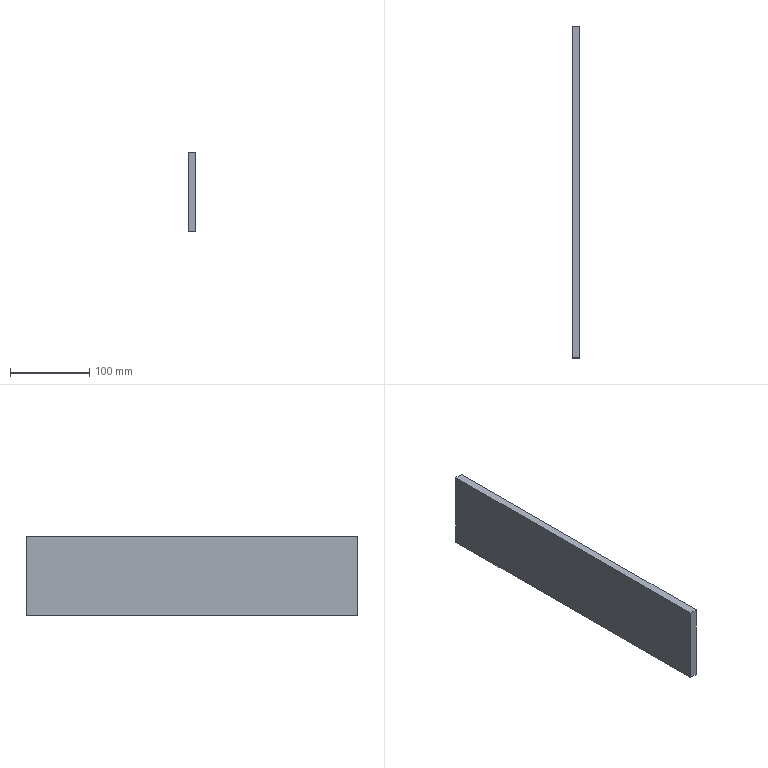Part | STEP file | PLA-AR | 1 solid | 206 faces | box 10 x 420 x 100 mm | volume 406379 mm3 | plane 206